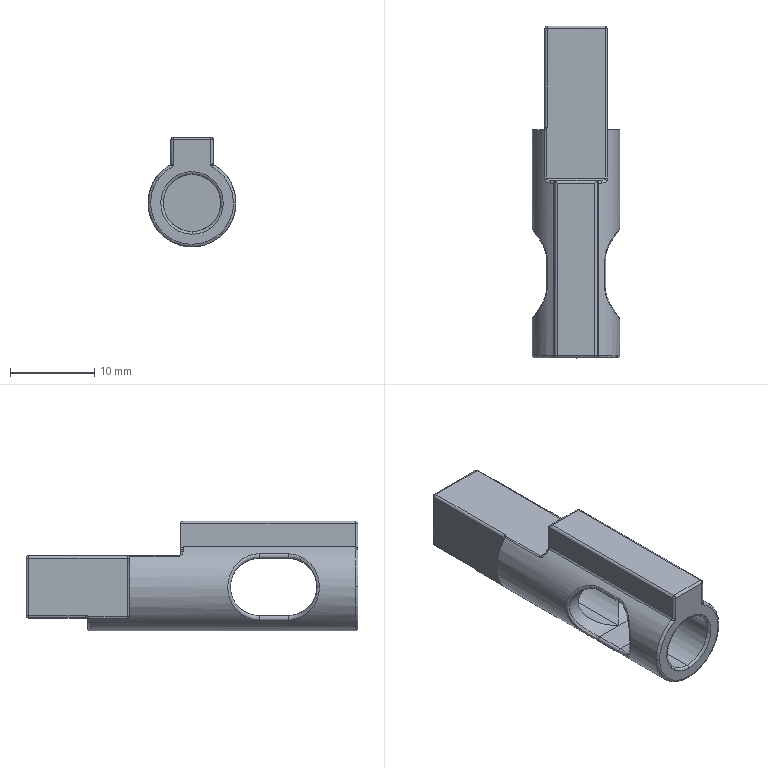Part | SolidWorks | features BaseBody 1 | 1 solid | 85 faces | box 10.402 x 39.3 x 13 mm | volume 2086 mm3 | cylinder 36 | plane 16 | spline 14 | torus 11 | sphere 8 | commonest cylinder face diameters 0.6 x26 6.8 x8 10.402 x2